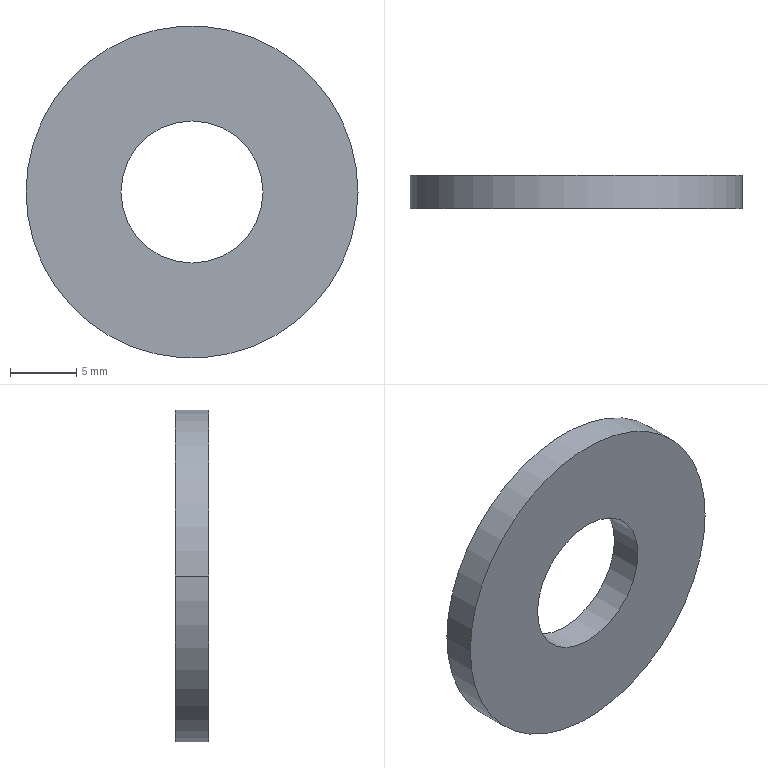Part | STEP file | M10_AALTOLAATTA_DIN125 | 1 solid | 6 faces | box 25 x 2.5 x 25 mm | volume 1002 mm3 | cylinder 4 | plane 2 | commonest cylinder face diameters 10.7 x2 25 x2
STEP:
#1=CARTESIAN_POINT('',(0.,0.,0.));
#2=DIRECTION('',(0.,0.,1.));
#3=DIRECTION('',(1.,0.,0.));
#4=AXIS2_PLACEMENT_3D('',#1,#2,#3);
#5=CARTESIAN_POINT('',(12.5,0.,0.));
#6=VERTEX_POINT('',#5);
#7=CARTESIAN_POINT('',(-12.5,0.,0.));
#8=VERTEX_POINT('',#7);
#9=CARTESIAN_POINT('',(0.,0.,0.));
#10=DIRECTION('',(0.,1.,0.));
#11=DIRECTION('',(1.,0.,0.));
#12=AXIS2_PLACEMENT_3D('',#9,#10,#11);
#13=CIRCLE('',#12,12.5);
#14=CARTESIAN_POINT('',(0.,0.,0.));
#15=DIRECTION('',(0.,1.,0.));
#16=DIRECTION('',(1.,0.,0.));
#17=AXIS2_PLACEMENT_3D('',#14,#15,#16);
#18=PLANE('',#17);
#19=CARTESIAN_POINT('',(0.,0.));
#20=DIRECTION('',(1.,0.));
#21=AXIS2_PLACEMENT_2D('',#19,#20);
#22=CIRCLE('',#21,12.5);
#23=(GEOMETRIC_REPRESENTATION_CONTEXT(2)PARAMETRIC_REPRESENTATION_CONTEXT()REPRESENTATION_CONTEXT('',''));
#24=DEFINITIONAL_REPRESENTATION('',(#22),#23);
#25=PCURVE('',#18,#24);
#26=CARTESIAN_POINT('',(0.,0.,0.));
#27=DIRECTION('',(0.,1.,0.));
#28=DIRECTION('',(1.,0.,0.));
#29=AXIS2_PLACEMENT_3D('',#26,#27,#28);
#30=CYLINDRICAL_SURFACE('',#29,12.5);
#31=CARTESIAN_POINT('',(0.,0.));
#32=DIRECTION('',(1.,0.));
#33=VECTOR('',#32,1.);
#34=LINE('',#31,#33);
#35=(GEOMETRIC_REPRESENTATION_CONTEXT(2)PARAMETRIC_REPRESENTATION_CONTEXT()REPRESENTATION_CONTEXT('',''));
#36=DEFINITIONAL_REPRESENTATION('',(#34),#35);
#37=PCURVE('',#30,#36);
#38=SURFACE_CURVE('',#13,(#25,#37),.PCURVE_S1.);
#39=EDGE_CURVE('',#6,#8,#38,.T.);
#40=ORIENTED_EDGE('',*,*,#39,.T.);
#41=CARTESIAN_POINT('',(0.,0.,0.));
#42=DIRECTION('',(0.,1.,0.));
#43=DIRECTION('',(-1.,0.,0.));
#44=AXIS2_PLACEMENT_3D('',#41,#42,#43);
#45=CIRCLE('',#44,12.5);
#46=CARTESIAN_POINT('',(0.,0.));
#47=DIRECTION('',(-1.,0.));
#48=AXIS2_PLACEMENT_2D('',#46,#47);
#49=CIRCLE('',#48,12.5);
#50=(GEOMETRIC_REPRESENTATION_CONTEXT(2)PARAMETRIC_REPRESENTATION_CONTEXT()REPRESENTATION_CONTEXT('',''));
#51=DEFINITIONAL_REPRESENTATION('',(#49),#50);
#52=PCURVE('',#18,#51);
#53=CARTESIAN_POINT('',(0.,0.,0.));
#54=DIRECTION('',(0.,1.,0.));
#55=DIRECTION('',(1.,0.,0.));
#56=AXIS2_PLACEMENT_3D('',#53,#54,#55);
#57=CYLINDRICAL_SURFACE('',#56,12.5);
#58=CARTESIAN_POINT('',(3.142,0.));
#59=DIRECTION('',(1.,0.));
#60=VECTOR('',#59,1.);
#61=LINE('',#58,#60);
#62=(GEOMETRIC_REPRESENTATION_CONTEXT(2)PARAMETRIC_REPRESENTATION_CONTEXT()REPRESENTATION_CONTEXT('',''));
#63=DEFINITIONAL_REPRESENTATION('',(#61),#62);
#64=PCURVE('',#57,#63);
#65=SURFACE_CURVE('',#45,(#52,#64),.PCURVE_S1.);
#66=EDGE_CURVE('',#8,#6,#65,.T.);
#67=ORIENTED_EDGE('',*,*,#66,.T.);
#68=EDGE_LOOP('',(#40,#67));
#69=FACE_BOUND('',#68,.F.);
#70=CARTESIAN_POINT('',(5.35,0.,0.));
#71=VERTEX_POINT('',#70);
#72=CARTESIAN_POINT('',(-5.35,0.,0.));
#73=VERTEX_POINT('',#72);
#74=CARTESIAN_POINT('',(0.,0.,0.));
#75=DIRECTION('',(0.,-1.,0.));
#76=DIRECTION('',(1.,0.,0.));
#77=AXIS2_PLACEMENT_3D('',#74,#75,#76);
#78=CIRCLE('',#77,5.35);
#79=CARTESIAN_POINT('',(5.35,0.));
#80=CARTESIAN_POINT('',(5.35,-9.266));
#81=CARTESIAN_POINT('',(-2.675,-4.633));
#82=CARTESIAN_POINT('',(-10.7,0.));
#83=CARTESIAN_POINT('',(-2.675,4.633));
#84=CARTESIAN_POINT('',(5.35,9.266));
#85=CARTESIAN_POINT('',(5.35,0.));
#86=(BOUNDED_CURVE()B_SPLINE_CURVE(2,(#79,#80,#81,#82,#83,#84,#85),.UNSPECIFIED.,.T.,.F.)B_SPLINE_CURVE_WITH_KNOTS((1,2,2,2,2,1),(-2.094,0.,2.094,4.189,6.283,8.378),.UNSPECIFIED.)CURVE()GEOMETRIC_REPRESENTATION_ITEM()RATIONAL_B_SPLINE_CURVE((1.,0.5,1.,0.5,1.,0.5,1.))REPRESENTATION_ITEM(''));
#87=(GEOMETRIC_REPRESENTATION_CONTEXT(2)PARAMETRIC_REPRESENTATION_CONTEXT()REPRESENTATION_CONTEXT('',''));
#88=DEFINITIONAL_REPRESENTATION('',(#86),#87);
#89=PCURVE('',#18,#88);
#90=CARTESIAN_POINT('',(0.,0.,0.));
#91=DIRECTION('',(0.,1.,0.));
#92=DIRECTION('',(1.,0.,0.));
#93=AXIS2_PLACEMENT_3D('',#90,#91,#92);
#94=CYLINDRICAL_SURFACE('',#93,5.35);
#95=CARTESIAN_POINT('',(6.283,0.));
#96=DIRECTION('',(-1.,0.));
#97=VECTOR('',#96,1.);
#98=LINE('',#95,#97);
#99=(GEOMETRIC_REPRESENTATION_CONTEXT(2)PARAMETRIC_REPRESENTATION_CONTEXT()REPRESENTATION_CONTEXT('',''));
#100=DEFINITIONAL_REPRESENTATION('',(#98),#99);
#101=PCURVE('',#94,#100);
#102=SURFACE_CURVE('',#78,(#89,#101),.PCURVE_S1.);
#103=EDGE_CURVE('',#71,#73,#102,.T.);
#104=ORIENTED_EDGE('',*,*,#103,.T.);
#105=CARTESIAN_POINT('',(0.,0.,0.));
#106=DIRECTION('',(0.,-1.,0.));
#107=DIRECTION('',(-1.,0.,0.));
#108=AXIS2_PLACEMENT_3D('',#105,#106,#107);
#109=CIRCLE('',#108,5.35);
#110=CARTESIAN_POINT('',(-5.35,0.));
#111=CARTESIAN_POINT('',(-5.35,9.266));
#112=CARTESIAN_POINT('',(2.675,4.633));
#113=CARTESIAN_POINT('',(10.7,0.));
#114=CARTESIAN_POINT('',(2.675,-4.633));
#115=CARTESIAN_POINT('',(-5.35,-9.266));
#116=CARTESIAN_POINT('',(-5.35,0.));
#117=(BOUNDED_CURVE()B_SPLINE_CURVE(2,(#110,#111,#112,#113,#114,#115,#116),.UNSPECIFIED.,.T.,.F.)B_SPLINE_CURVE_WITH_KNOTS((1,2,2,2,2,1),(-2.094,0.,2.094,4.189,6.283,8.378),.UNSPECIFIED.)CURVE()GEOMETRIC_REPRESENTATION_ITEM()RATIONAL_B_SPLINE_CURVE((1.,0.5,1.,0.5,1.,0.5,1.))REPRESENTATION_ITEM(''));
#118=(GEOMETRIC_REPRESENTATION_CONTEXT(2)PARAMETRIC_REPRESENTATION_CONTEXT()REPRESENTATION_CONTEXT('',''));
#119=DEFINITIONAL_REPRESENTATION('',(#117),#118);
#120=PCURVE('',#18,#119);
#121=CARTESIAN_POINT('',(0.,0.,0.));
#122=DIRECTION('',(0.,1.,0.));
#123=DIRECTION('',(1.,0.,0.));
#124=AXIS2_PLACEMENT_3D('',#121,#122,#123);
#125=CYLINDRICAL_SURFACE('',#124,5.35);
#126=CARTESIAN_POINT('',(3.142,0.));
#127=DIRECTION('',(-1.,0.));
#128=VECTOR('',#127,1.);
#129=LINE('',#126,#128);
#130=(GEOMETRIC_REPRESENTATION_CONTEXT(2)PARAMETRIC_REPRESENTATION_CONTEXT()REPRESENTATION_CONTEXT('',''));
#131=DEFINITIONAL_REPRESENTATION('',(#129),#130);
#132=PCURVE('',#125,#131);
#133=SURFACE_CURVE('',#109,(#120,#132),.PCURVE_S1.);
#134=EDGE_CURVE('',#73,#71,#133,.T.);
#135=ORIENTED_EDGE('',*,*,#134,.T.);
#136=EDGE_LOOP('',(#104,#135));
#137=FACE_BOUND('',#136,.F.);
#138=ADVANCED_FACE('',(#69,#137),#18,.F.);
#139=CARTESIAN_POINT('',(-12.5,2.5,0.));
#140=VERTEX_POINT('',#139);
#141=CARTESIAN_POINT('',(-12.5,0.,0.));
#142=DIRECTION('',(0.,1.,0.));
#143=VECTOR('',#142,1.);
#144=LINE('',#141,#143);
#145=CARTESIAN_POINT('',(3.142,0.));
#146=DIRECTION('',(0.,1.));
#147=VECTOR('',#146,1.);
#148=LINE('',#145,#147);
#149=(GEOMETRIC_REPRESENTATION_CONTEXT(2)PARAMETRIC_REPRESENTATION_CONTEXT()REPRESENTATION_CONTEXT('',''));
#150=DEFINITIONAL_REPRESENTATION('',(#148),#149);
#151=PCURVE('',#30,#150);
#152=CARTESIAN_POINT('',(3.142,0.));
#153=DIRECTION('',(0.,1.));
#154=VECTOR('',#153,1.);
#155=LINE('',#152,#154);
#156=(GEOMETRIC_REPRESENTATION_CONTEXT(2)PARAMETRIC_REPRESENTATION_CONTEXT()REPRESENTATION_CONTEXT('',''));
#157=DEFINITIONAL_REPRESENTATION('',(#155),#156);
#158=PCURVE('',#57,#157);
#159=SURFACE_CURVE('',#144,(#151,#158),.PCURVE_S1.);
#160=EDGE_CURVE('',#8,#140,#159,.T.);
#161=ORIENTED_EDGE('',*,*,#160,.T.);
#162=CARTESIAN_POINT('',(12.5,2.5,0.));
#163=VERTEX_POINT('',#162);
#164=CARTESIAN_POINT('',(0.,2.5,0.));
#165=DIRECTION('',(0.,1.,0.));
#166=DIRECTION('',(1.,0.,0.));
#167=AXIS2_PLACEMENT_3D('',#164,#165,#166);
#168=CIRCLE('',#167,12.5);
#169=CARTESIAN_POINT('',(0.,2.5));
#170=DIRECTION('',(1.,0.));
#171=VECTOR('',#170,1.);
#172=LINE('',#169,#171);
#173=(GEOMETRIC_REPRESENTATION_CONTEXT(2)PARAMETRIC_REPRESENTATION_CONTEXT()REPRESENTATION_CONTEXT('',''));
#174=DEFINITIONAL_REPRESENTATION('',(#172),#173);
#175=PCURVE('',#30,#174);
#176=CARTESIAN_POINT('',(0.,2.5,0.));
#177=DIRECTION('',(0.,1.,0.));
#178=DIRECTION('',(1.,0.,0.));
#179=AXIS2_PLACEMENT_3D('',#176,#177,#178);
#180=PLANE('',#179);
#181=CARTESIAN_POINT('',(0.,0.));
#182=DIRECTION('',(1.,0.));
#183=AXIS2_PLACEMENT_2D('',#181,#182);
#184=CIRCLE('',#183,12.5);
#185=(GEOMETRIC_REPRESENTATION_CONTEXT(2)PARAMETRIC_REPRESENTATION_CONTEXT()REPRESENTATION_CONTEXT('',''));
#186=DEFINITIONAL_REPRESENTATION('',(#184),#185);
#187=PCURVE('',#180,#186);
#188=SURFACE_CURVE('',#168,(#175,#187),.PCURVE_S1.);
#189=EDGE_CURVE('',#163,#140,#188,.T.);
#190=ORIENTED_EDGE('',*,*,#189,.F.);
#191=CARTESIAN_POINT('',(12.5,0.,0.));
#192=DIRECTION('',(0.,1.,0.));
#193=VECTOR('',#192,1.);
#194=LINE('',#191,#193);
#195=CARTESIAN_POINT('',(0.,0.));
#196=DIRECTION('',(0.,1.));
#197=VECTOR('',#196,1.);
#198=LINE('',#195,#197);
#199=(GEOMETRIC_REPRESENTATION_CONTEXT(2)PARAMETRIC_REPRESENTATION_CONTEXT()REPRESENTATION_CONTEXT('',''));
#200=DEFINITIONAL_REPRESENTATION('',(#198),#199);
#201=PCURVE('',#30,#200);
#202=CARTESIAN_POINT('',(6.283,0.));
#203=DIRECTION('',(0.,1.));
#204=VECTOR('',#203,1.);
#205=LINE('',#202,#204);
#206=(GEOMETRIC_REPRESENTATION_CONTEXT(2)PARAMETRIC_REPRESENTATION_CONTEXT()REPRESENTATION_CONTEXT('',''));
#207=DEFINITIONAL_REPRESENTATION('',(#205),#206);
#208=PCURVE('',#57,#207);
#209=SURFACE_CURVE('',#194,(#201,#208),.PCURVE_S1.);
#210=EDGE_CURVE('',#6,#163,#209,.T.);
#211=ORIENTED_EDGE('',*,*,#210,.F.);
#212=ORIENTED_EDGE('',*,*,#39,.T.);
#213=EDGE_LOOP('',(#161,#190,#211,#212));
#214=FACE_BOUND('',#213,.T.);
#215=ADVANCED_FACE('',(#214),#30,.T.);
#216=ORIENTED_EDGE('',*,*,#210,.T.);
#217=CARTESIAN_POINT('',(0.,2.5,0.));
#218=DIRECTION('',(0.,1.,0.));
#219=DIRECTION('',(-1.,0.,0.));
#220=AXIS2_PLACEMENT_3D('',#217,#218,#219);
#221=CIRCLE('',#220,12.5);
#222=CARTESIAN_POINT('',(3.142,2.5));
#223=DIRECTION('',(1.,0.));
#224=VECTOR('',#223,1.);
#225=LINE('',#222,#224);
#226=(GEOMETRIC_REPRESENTATION_CONTEXT(2)PARAMETRIC_REPRESENTATION_CONTEXT()REPRESENTATION_CONTEXT('',''));
#227=DEFINITIONAL_REPRESENTATION('',(#225),#226);
#228=PCURVE('',#57,#227);
#229=CARTESIAN_POINT('',(0.,0.));
#230=DIRECTION('',(-1.,0.));
#231=AXIS2_PLACEMENT_2D('',#229,#230);
#232=CIRCLE('',#231,12.5);
#233=(GEOMETRIC_REPRESENTATION_CONTEXT(2)PARAMETRIC_REPRESENTATION_CONTEXT()REPRESENTATION_CONTEXT('',''));
#234=DEFINITIONAL_REPRESENTATION('',(#232),#233);
#235=PCURVE('',#180,#234);
#236=SURFACE_CURVE('',#221,(#228,#235),.PCURVE_S1.);
#237=EDGE_CURVE('',#140,#163,#236,.T.);
#238=ORIENTED_EDGE('',*,*,#237,.F.);
#239=ORIENTED_EDGE('',*,*,#160,.F.);
#240=ORIENTED_EDGE('',*,*,#66,.T.);
#241=EDGE_LOOP('',(#216,#238,#239,#240));
#242=FACE_BOUND('',#241,.T.);
#243=ADVANCED_FACE('',(#242),#57,.T.);
#244=ORIENTED_EDGE('',*,*,#189,.F.);
#245=ORIENTED_EDGE('',*,*,#237,.F.);
#246=EDGE_LOOP('',(#244,#245));
#247=FACE_BOUND('',#246,.F.);
#248=CARTESIAN_POINT('',(5.35,2.5,0.));
#249=VERTEX_POINT('',#248);
#250=CARTESIAN_POINT('',(-5.35,2.5,0.));
#251=VERTEX_POINT('',#250);
#252=CARTESIAN_POINT('',(0.,2.5,0.));
#253=DIRECTION('',(0.,-1.,0.));
#254=DIRECTION('',(1.,0.,0.));
#255=AXIS2_PLACEMENT_3D('',#252,#253,#254);
#256=CIRCLE('',#255,5.35);
#257=CARTESIAN_POINT('',(5.35,0.));
#258=CARTESIAN_POINT('',(5.35,-9.266));
#259=CARTESIAN_POINT('',(-2.675,-4.633));
#260=CARTESIAN_POINT('',(-10.7,0.));
#261=CARTESIAN_POINT('',(-2.675,4.633));
#262=CARTESIAN_POINT('',(5.35,9.266));
#263=CARTESIAN_POINT('',(5.35,0.));
#264=(BOUNDED_CURVE()B_SPLINE_CURVE(2,(#257,#258,#259,#260,#261,#262,#263),.UNSPECIFIED.,.T.,.F.)B_SPLINE_CURVE_WITH_KNOTS((1,2,2,2,2,1),(-2.094,0.,2.094,4.189,6.283,8.378),.UNSPECIFIED.)CURVE()GEOMETRIC_REPRESENTATION_ITEM()RATIONAL_B_SPLINE_CURVE((1.,0.5,1.,0.5,1.,0.5,1.))REPRESENTATION_ITEM(''));
#265=(GEOMETRIC_REPRESENTATION_CONTEXT(2)PARAMETRIC_REPRESENTATION_CONTEXT()REPRESENTATION_CONTEXT('',''));
#266=DEFINITIONAL_REPRESENTATION('',(#264),#265);
#267=PCURVE('',#180,#266);
#268=CARTESIAN_POINT('',(6.283,2.5));
#269=DIRECTION('',(-1.,0.));
#270=VECTOR('',#269,1.);
#271=LINE('',#268,#270);
#272=(GEOMETRIC_REPRESENTATION_CONTEXT(2)PARAMETRIC_REPRESENTATION_CONTEXT()REPRESENTATION_CONTEXT('',''));
#273=DEFINITIONAL_REPRESENTATION('',(#271),#272);
#274=PCURVE('',#94,#273);
#275=SURFACE_CURVE('',#256,(#267,#274),.PCURVE_S1.);
#276=EDGE_CURVE('',#249,#251,#275,.T.);
#277=ORIENTED_EDGE('',*,*,#276,.F.);
#278=CARTESIAN_POINT('',(0.,2.5,0.));
#279=DIRECTION('',(0.,-1.,0.));
#280=DIRECTION('',(-1.,0.,0.));
#281=AXIS2_PLACEMENT_3D('',#278,#279,#280);
#282=CIRCLE('',#281,5.35);
#283=CARTESIAN_POINT('',(-5.35,0.));
#284=CARTESIAN_POINT('',(-5.35,9.266));
#285=CARTESIAN_POINT('',(2.675,4.633));
#286=CARTESIAN_POINT('',(10.7,0.));
#287=CARTESIAN_POINT('',(2.675,-4.633));
#288=CARTESIAN_POINT('',(-5.35,-9.266));
#289=CARTESIAN_POINT('',(-5.35,0.));
#290=(BOUNDED_CURVE()B_SPLINE_CURVE(2,(#283,#284,#285,#286,#287,#288,#289),.UNSPECIFIED.,.T.,.F.)B_SPLINE_CURVE_WITH_KNOTS((1,2,2,2,2,1),(-2.094,0.,2.094,4.189,6.283,8.378),.UNSPECIFIED.)CURVE()GEOMETRIC_REPRESENTATION_ITEM()RATIONAL_B_SPLINE_CURVE((1.,0.5,1.,0.5,1.,0.5,1.))REPRESENTATION_ITEM(''));
#291=(GEOMETRIC_REPRESENTATION_CONTEXT(2)PARAMETRIC_REPRESENTATION_CONTEXT()REPRESENTATION_CONTEXT('',''));
#292=DEFINITIONAL_REPRESENTATION('',(#290),#291);
#293=PCURVE('',#180,#292);
#294=CARTESIAN_POINT('',(3.142,2.5));
#295=DIRECTION('',(-1.,0.));
#296=VECTOR('',#295,1.);
#297=LINE('',#294,#296);
#298=(GEOMETRIC_REPRESENTATION_CONTEXT(2)PARAMETRIC_REPRESENTATION_CONTEXT()REPRESENTATION_CONTEXT('',''));
#299=DEFINITIONAL_REPRESENTATION('',(#297),#298);
#300=PCURVE('',#125,#299);
#301=SURFACE_CURVE('',#282,(#293,#300),.PCURVE_S1.);
#302=EDGE_CURVE('',#251,#249,#301,.T.);
#303=ORIENTED_EDGE('',*,*,#302,.F.);
#304=EDGE_LOOP('',(#277,#303));
#305=FACE_BOUND('',#304,.F.);
#306=ADVANCED_FACE('',(#247,#305),#180,.T.);
#307=ORIENTED_EDGE('',*,*,#103,.F.);
#308=CARTESIAN_POINT('',(5.35,0.,0.));
#309=DIRECTION('',(0.,1.,0.));
#310=VECTOR('',#309,1.);
#311=LINE('',#308,#310);
#312=CARTESIAN_POINT('',(6.283,0.));
#313=DIRECTION('',(0.,1.));
#314=VECTOR('',#313,1.);
#315=LINE('',#312,#314);
#316=(GEOMETRIC_REPRESENTATION_CONTEXT(2)PARAMETRIC_REPRESENTATION_CONTEXT()REPRESENTATION_CONTEXT('',''));
#317=DEFINITIONAL_REPRESENTATION('',(#315),#316);
#318=PCURVE('',#94,#317);
#319=CARTESIAN_POINT('',(0.,0.));
#320=DIRECTION('',(0.,1.));
#321=VECTOR('',#320,1.);
#322=LINE('',#319,#321);
#323=(GEOMETRIC_REPRESENTATION_CONTEXT(2)PARAMETRIC_REPRESENTATION_CONTEXT()REPRESENTATION_CONTEXT('',''));
#324=DEFINITIONAL_REPRESENTATION('',(#322),#323);
#325=PCURVE('',#125,#324);
#326=SURFACE_CURVE('',#311,(#318,#325),.PCURVE_S1.);
#327=EDGE_CURVE('',#71,#249,#326,.T.);
#328=ORIENTED_EDGE('',*,*,#327,.T.);
#329=ORIENTED_EDGE('',*,*,#276,.T.);
#330=CARTESIAN_POINT('',(-5.35,0.,0.));
#331=DIRECTION('',(0.,1.,0.));
#332=VECTOR('',#331,1.);
#333=LINE('',#330,#332);
#334=CARTESIAN_POINT('',(3.142,0.));
#335=DIRECTION('',(0.,1.));
#336=VECTOR('',#335,1.);
#337=LINE('',#334,#336);
#338=(GEOMETRIC_REPRESENTATION_CONTEXT(2)PARAMETRIC_REPRESENTATION_CONTEXT()REPRESENTATION_CONTEXT('',''));
#339=DEFINITIONAL_REPRESENTATION('',(#337),#338);
#340=PCURVE('',#94,#339);
#341=CARTESIAN_POINT('',(3.142,0.));
#342=DIRECTION('',(0.,1.));
#343=VECTOR('',#342,1.);
#344=LINE('',#341,#343);
#345=(GEOMETRIC_REPRESENTATION_CONTEXT(2)PARAMETRIC_REPRESENTATION_CONTEXT()REPRESENTATION_CONTEXT('',''));
#346=DEFINITIONAL_REPRESENTATION('',(#344),#345);
#347=PCURVE('',#125,#346);
#348=SURFACE_CURVE('',#333,(#340,#347),.PCURVE_S1.);
#349=EDGE_CURVE('',#73,#251,#348,.T.);
#350=ORIENTED_EDGE('',*,*,#349,.F.);
#351=EDGE_LOOP('',(#307,#328,#329,#350));
#352=FACE_BOUND('',#351,.F.);
#353=ADVANCED_FACE('',(#352),#94,.F.);
#354=ORIENTED_EDGE('',*,*,#134,.F.);
#355=ORIENTED_EDGE('',*,*,#349,.T.);
#356=ORIENTED_EDGE('',*,*,#302,.T.);
#357=ORIENTED_EDGE('',*,*,#327,.F.);
#358=EDGE_LOOP('',(#354,#355,#356,#357));
#359=FACE_BOUND('',#358,.F.);
#360=ADVANCED_FACE('',(#359),#125,.F.);
#361=CLOSED_SHELL('',(#138,#215,#243,#306,#353,#360));
#362=MANIFOLD_SOLID_BREP('',#361);
#363=(LENGTH_UNIT()NAMED_UNIT(*)SI_UNIT(.MILLI.,.METRE.));
#364=UNCERTAINTY_MEASURE_WITH_UNIT(LENGTH_MEASURE(0.0000001),#363,'','');
#365=(NAMED_UNIT(*)PLANE_ANGLE_UNIT()SI_UNIT($,.RADIAN.));
#366=(NAMED_UNIT(*)SI_UNIT($,.STERADIAN.)SOLID_ANGLE_UNIT());
#367=(GEOMETRIC_REPRESENTATION_CONTEXT(3)GLOBAL_UNCERTAINTY_ASSIGNED_CONTEXT((#364))GLOBAL_UNIT_ASSIGNED_CONTEXT((#363,#365,#366))REPRESENTATION_CONTEXT('',''));
#368=ADVANCED_BREP_SHAPE_REPRESENTATION('',(#4,#362),#367);